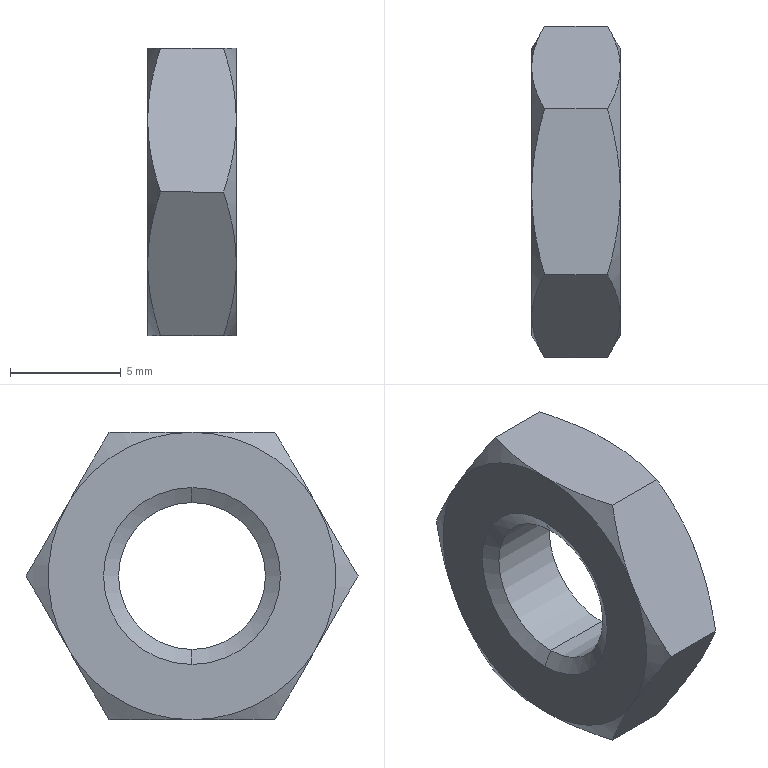Part | STEP file | 0217_306_SNTRCS8 | 1 solid | 26 faces | box 4 x 15.011 x 13 mm | volume 435.9 mm3 | cone 16 | plane 8 | cylinder 2 | commonest cylinder face diameters 6.647 x2